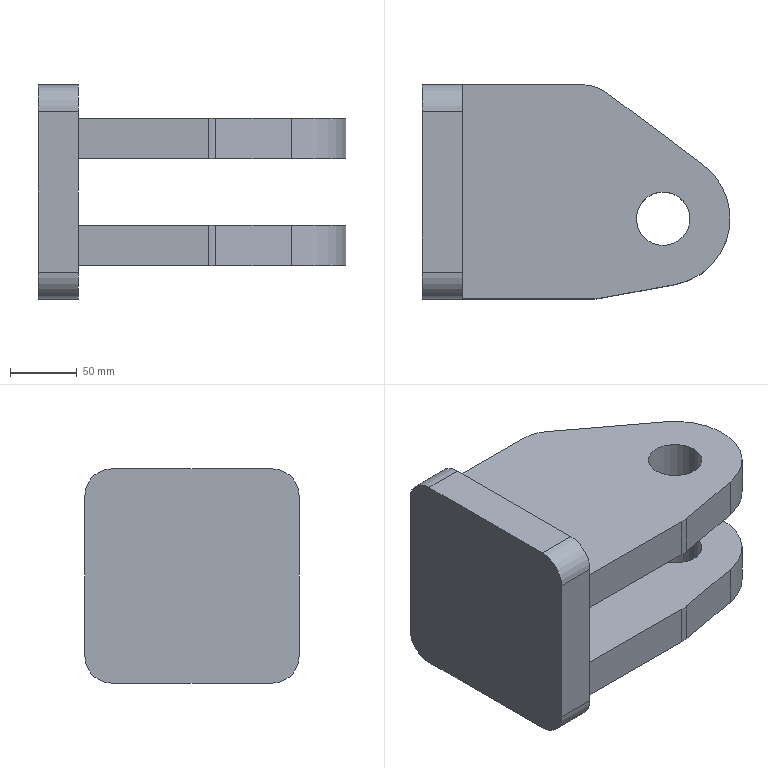Part | SolidWorks | features BaseBody 3 | 3 solids | 34 faces | box 230 x 160 x 160 mm | volume 2295420 mm3 | plane 20 | cylinder 14 | commonest cylinder face diameters 40 x8 60 x4 100 x2
STEP:
#1=CARTESIAN_POINT('',(-15.,60.,-80.));
#2=VERTEX_POINT('',#1);
#3=CARTESIAN_POINT('',(-15.,80.,-60.));
#4=VERTEX_POINT('',#3);
#5=CARTESIAN_POINT('',(-15.,60.,-60.));
#6=DIRECTION('',(1.,0.,0.));
#7=DIRECTION('',(0.,0.,1.));
#8=AXIS2_PLACEMENT_3D('',#5,#6,#7);
#9=CIRCLE('',#8,20.);
#10=EDGE_CURVE('',#2,#4,#9,.T.);
#11=ORIENTED_EDGE('',*,*,#10,.T.);
#12=CARTESIAN_POINT('',(15.,80.,-60.));
#13=VERTEX_POINT('',#12);
#14=CARTESIAN_POINT('',(15.,80.,-60.));
#15=DIRECTION('',(-1.,0.,0.));
#16=VECTOR('',#15,1000.);
#17=LINE('',#14,#16);
#18=EDGE_CURVE('',#13,#4,#17,.T.);
#19=ORIENTED_EDGE('',*,*,#18,.F.);
#20=CARTESIAN_POINT('',(15.,60.,-80.));
#21=VERTEX_POINT('',#20);
#22=CARTESIAN_POINT('',(15.,60.,-60.));
#23=DIRECTION('',(1.,0.,0.));
#24=DIRECTION('',(0.,0.,1.));
#25=AXIS2_PLACEMENT_3D('',#22,#23,#24);
#26=CIRCLE('',#25,20.);
#27=EDGE_CURVE('',#21,#13,#26,.T.);
#28=ORIENTED_EDGE('',*,*,#27,.F.);
#29=CARTESIAN_POINT('',(15.,60.,-80.));
#30=DIRECTION('',(-1.,0.,0.));
#31=VECTOR('',#30,1000.);
#32=LINE('',#29,#31);
#33=EDGE_CURVE('',#21,#2,#32,.T.);
#34=ORIENTED_EDGE('',*,*,#33,.T.);
#35=EDGE_LOOP('',(#11,#19,#28,#34));
#36=FACE_OUTER_BOUND('',#35,.T.);
#37=CARTESIAN_POINT('',(15.,60.,-60.));
#38=DIRECTION('',(-1.,0.,0.));
#39=DIRECTION('',(0.,0.,1.));
#40=AXIS2_PLACEMENT_3D('',#37,#38,#39);
#41=CYLINDRICAL_SURFACE('',#40,20.);
#42=ADVANCED_FACE('',(#36),#41,.T.);
#43=CARTESIAN_POINT('',(-15.,80.,60.));
#44=VERTEX_POINT('',#43);
#45=CARTESIAN_POINT('',(-15.,80.,60.));
#46=DIRECTION('',(0.,0.,1.));
#47=VECTOR('',#46,1000.);
#48=LINE('',#45,#47);
#49=EDGE_CURVE('',#4,#44,#48,.T.);
#50=ORIENTED_EDGE('',*,*,#49,.T.);
#51=CARTESIAN_POINT('',(15.,80.,60.));
#52=VERTEX_POINT('',#51);
#53=CARTESIAN_POINT('',(15.,80.,60.));
#54=DIRECTION('',(-1.,0.,0.));
#55=VECTOR('',#54,1000.);
#56=LINE('',#53,#55);
#57=EDGE_CURVE('',#52,#44,#56,.T.);
#58=ORIENTED_EDGE('',*,*,#57,.F.);
#59=CARTESIAN_POINT('',(15.,80.,60.));
#60=DIRECTION('',(0.,0.,1.));
#61=VECTOR('',#60,1000.);
#62=LINE('',#59,#61);
#63=EDGE_CURVE('',#13,#52,#62,.T.);
#64=ORIENTED_EDGE('',*,*,#63,.F.);
#65=ORIENTED_EDGE('',*,*,#18,.T.);
#66=EDGE_LOOP('',(#50,#58,#64,#65));
#67=FACE_OUTER_BOUND('',#66,.T.);
#68=CARTESIAN_POINT('',(15.,80.,60.));
#69=DIRECTION('',(0.,-1.,0.));
#70=DIRECTION('',(0.,0.,-1.));
#71=AXIS2_PLACEMENT_3D('',#68,#69,#70);
#72=PLANE('',#71);
#73=ADVANCED_FACE('',(#67),#72,.F.);
#74=CARTESIAN_POINT('',(-15.,60.,80.));
#75=VERTEX_POINT('',#74);
#76=CARTESIAN_POINT('',(-15.,60.,60.));
#77=DIRECTION('',(1.,0.,0.));
#78=DIRECTION('',(0.,0.,-1.));
#79=AXIS2_PLACEMENT_3D('',#76,#77,#78);
#80=CIRCLE('',#79,20.);
#81=EDGE_CURVE('',#44,#75,#80,.T.);
#82=ORIENTED_EDGE('',*,*,#81,.T.);
#83=CARTESIAN_POINT('',(15.,60.,80.));
#84=VERTEX_POINT('',#83);
#85=CARTESIAN_POINT('',(15.,60.,80.));
#86=DIRECTION('',(-1.,0.,0.));
#87=VECTOR('',#86,1000.);
#88=LINE('',#85,#87);
#89=EDGE_CURVE('',#84,#75,#88,.T.);
#90=ORIENTED_EDGE('',*,*,#89,.F.);
#91=CARTESIAN_POINT('',(15.,60.,60.));
#92=DIRECTION('',(1.,0.,0.));
#93=DIRECTION('',(0.,0.,-1.));
#94=AXIS2_PLACEMENT_3D('',#91,#92,#93);
#95=CIRCLE('',#94,20.);
#96=EDGE_CURVE('',#52,#84,#95,.T.);
#97=ORIENTED_EDGE('',*,*,#96,.F.);
#98=ORIENTED_EDGE('',*,*,#57,.T.);
#99=EDGE_LOOP('',(#82,#90,#97,#98));
#100=FACE_OUTER_BOUND('',#99,.T.);
#101=CARTESIAN_POINT('',(15.,60.,60.));
#102=DIRECTION('',(-1.,0.,0.));
#103=DIRECTION('',(0.,0.,1.));
#104=AXIS2_PLACEMENT_3D('',#101,#102,#103);
#105=CYLINDRICAL_SURFACE('',#104,20.);
#106=ADVANCED_FACE('',(#100),#105,.T.);
#107=CARTESIAN_POINT('',(-15.,-60.,80.));
#108=VERTEX_POINT('',#107);
#109=CARTESIAN_POINT('',(-15.,60.,80.));
#110=DIRECTION('',(0.,-1.,0.));
#111=VECTOR('',#110,1000.);
#112=LINE('',#109,#111);
#113=EDGE_CURVE('',#75,#108,#112,.T.);
#114=ORIENTED_EDGE('',*,*,#113,.T.);
#115=CARTESIAN_POINT('',(15.,-60.,80.));
#116=VERTEX_POINT('',#115);
#117=CARTESIAN_POINT('',(15.,-60.,80.));
#118=DIRECTION('',(-1.,0.,0.));
#119=VECTOR('',#118,1000.);
#120=LINE('',#117,#119);
#121=EDGE_CURVE('',#116,#108,#120,.T.);
#122=ORIENTED_EDGE('',*,*,#121,.F.);
#123=CARTESIAN_POINT('',(15.,60.,80.));
#124=DIRECTION('',(0.,-1.,0.));
#125=VECTOR('',#124,1000.);
#126=LINE('',#123,#125);
#127=EDGE_CURVE('',#84,#116,#126,.T.);
#128=ORIENTED_EDGE('',*,*,#127,.F.);
#129=ORIENTED_EDGE('',*,*,#89,.T.);
#130=EDGE_LOOP('',(#114,#122,#128,#129));
#131=FACE_OUTER_BOUND('',#130,.T.);
#132=CARTESIAN_POINT('',(15.,60.,80.));
#133=DIRECTION('',(0.,0.,-1.));
#134=DIRECTION('',(-1.,0.,0.));
#135=AXIS2_PLACEMENT_3D('',#132,#133,#134);
#136=PLANE('',#135);
#137=ADVANCED_FACE('',(#131),#136,.F.);
#138=CARTESIAN_POINT('',(-15.,-80.,60.));
#139=VERTEX_POINT('',#138);
#140=CARTESIAN_POINT('',(-15.,-60.,60.));
#141=DIRECTION('',(1.,0.,0.));
#142=DIRECTION('',(0.,0.,-1.));
#143=AXIS2_PLACEMENT_3D('',#140,#141,#142);
#144=CIRCLE('',#143,20.);
#145=EDGE_CURVE('',#108,#139,#144,.T.);
#146=ORIENTED_EDGE('',*,*,#145,.T.);
#147=CARTESIAN_POINT('',(15.,-80.,60.));
#148=VERTEX_POINT('',#147);
#149=CARTESIAN_POINT('',(15.,-80.,60.));
#150=DIRECTION('',(-1.,0.,0.));
#151=VECTOR('',#150,1000.);
#152=LINE('',#149,#151);
#153=EDGE_CURVE('',#148,#139,#152,.T.);
#154=ORIENTED_EDGE('',*,*,#153,.F.);
#155=CARTESIAN_POINT('',(15.,-60.,60.));
#156=DIRECTION('',(1.,0.,0.));
#157=DIRECTION('',(0.,0.,-1.));
#158=AXIS2_PLACEMENT_3D('',#155,#156,#157);
#159=CIRCLE('',#158,20.);
#160=EDGE_CURVE('',#116,#148,#159,.T.);
#161=ORIENTED_EDGE('',*,*,#160,.F.);
#162=ORIENTED_EDGE('',*,*,#121,.T.);
#163=EDGE_LOOP('',(#146,#154,#161,#162));
#164=FACE_OUTER_BOUND('',#163,.T.);
#165=CARTESIAN_POINT('',(15.,-60.,60.));
#166=DIRECTION('',(-1.,0.,0.));
#167=DIRECTION('',(0.,0.,1.));
#168=AXIS2_PLACEMENT_3D('',#165,#166,#167);
#169=CYLINDRICAL_SURFACE('',#168,20.);
#170=ADVANCED_FACE('',(#164),#169,.T.);
#171=CARTESIAN_POINT('',(-15.,-80.,-60.));
#172=VERTEX_POINT('',#171);
#173=CARTESIAN_POINT('',(-15.,-80.,60.));
#174=DIRECTION('',(0.,0.,-1.));
#175=VECTOR('',#174,1000.);
#176=LINE('',#173,#175);
#177=EDGE_CURVE('',#139,#172,#176,.T.);
#178=ORIENTED_EDGE('',*,*,#177,.T.);
#179=CARTESIAN_POINT('',(15.,-80.,-60.));
#180=VERTEX_POINT('',#179);
#181=CARTESIAN_POINT('',(15.,-80.,-60.));
#182=DIRECTION('',(-1.,0.,0.));
#183=VECTOR('',#182,1000.);
#184=LINE('',#181,#183);
#185=EDGE_CURVE('',#180,#172,#184,.T.);
#186=ORIENTED_EDGE('',*,*,#185,.F.);
#187=CARTESIAN_POINT('',(15.,-80.,60.));
#188=DIRECTION('',(0.,0.,-1.));
#189=VECTOR('',#188,1000.);
#190=LINE('',#187,#189);
#191=EDGE_CURVE('',#148,#180,#190,.T.);
#192=ORIENTED_EDGE('',*,*,#191,.F.);
#193=ORIENTED_EDGE('',*,*,#153,.T.);
#194=EDGE_LOOP('',(#178,#186,#192,#193));
#195=FACE_OUTER_BOUND('',#194,.T.);
#196=CARTESIAN_POINT('',(15.,-80.,60.));
#197=DIRECTION('',(0.,1.,0.));
#198=DIRECTION('',(0.,0.,1.));
#199=AXIS2_PLACEMENT_3D('',#196,#197,#198);
#200=PLANE('',#199);
#201=ADVANCED_FACE('',(#195),#200,.F.);
#202=CARTESIAN_POINT('',(-15.,-60.,-80.));
#203=VERTEX_POINT('',#202);
#204=CARTESIAN_POINT('',(-15.,-60.,-60.));
#205=DIRECTION('',(1.,0.,0.));
#206=DIRECTION('',(0.,0.,-1.));
#207=AXIS2_PLACEMENT_3D('',#204,#205,#206);
#208=CIRCLE('',#207,20.);
#209=EDGE_CURVE('',#172,#203,#208,.T.);
#210=ORIENTED_EDGE('',*,*,#209,.T.);
#211=CARTESIAN_POINT('',(15.,-60.,-80.));
#212=VERTEX_POINT('',#211);
#213=CARTESIAN_POINT('',(15.,-60.,-80.));
#214=DIRECTION('',(-1.,0.,0.));
#215=VECTOR('',#214,1000.);
#216=LINE('',#213,#215);
#217=EDGE_CURVE('',#212,#203,#216,.T.);
#218=ORIENTED_EDGE('',*,*,#217,.F.);
#219=CARTESIAN_POINT('',(15.,-60.,-60.));
#220=DIRECTION('',(1.,0.,0.));
#221=DIRECTION('',(0.,0.,-1.));
#222=AXIS2_PLACEMENT_3D('',#219,#220,#221);
#223=CIRCLE('',#222,20.);
#224=EDGE_CURVE('',#180,#212,#223,.T.);
#225=ORIENTED_EDGE('',*,*,#224,.F.);
#226=ORIENTED_EDGE('',*,*,#185,.T.);
#227=EDGE_LOOP('',(#210,#218,#225,#226));
#228=FACE_OUTER_BOUND('',#227,.T.);
#229=CARTESIAN_POINT('',(15.,-60.,-60.));
#230=DIRECTION('',(-1.,0.,0.));
#231=DIRECTION('',(0.,0.,1.));
#232=AXIS2_PLACEMENT_3D('',#229,#230,#231);
#233=CYLINDRICAL_SURFACE('',#232,20.);
#234=ADVANCED_FACE('',(#228),#233,.T.);
#235=CARTESIAN_POINT('',(-15.,60.,-80.));
#236=DIRECTION('',(0.,1.,0.));
#237=VECTOR('',#236,1000.);
#238=LINE('',#235,#237);
#239=EDGE_CURVE('',#203,#2,#238,.T.);
#240=ORIENTED_EDGE('',*,*,#239,.T.);
#241=ORIENTED_EDGE('',*,*,#33,.F.);
#242=CARTESIAN_POINT('',(15.,60.,-80.));
#243=DIRECTION('',(0.,1.,0.));
#244=VECTOR('',#243,1000.);
#245=LINE('',#242,#244);
#246=EDGE_CURVE('',#212,#21,#245,.T.);
#247=ORIENTED_EDGE('',*,*,#246,.F.);
#248=ORIENTED_EDGE('',*,*,#217,.T.);
#249=EDGE_LOOP('',(#240,#241,#247,#248));
#250=FACE_OUTER_BOUND('',#249,.T.);
#251=CARTESIAN_POINT('',(15.,60.,-80.));
#252=DIRECTION('',(0.,0.,1.));
#253=DIRECTION('',(0.,-1.,0.));
#254=AXIS2_PLACEMENT_3D('',#251,#252,#253);
#255=PLANE('',#254);
#256=ADVANCED_FACE('',(#250),#255,.F.);
#257=ORIENTED_EDGE('',*,*,#27,.T.);
#258=ORIENTED_EDGE('',*,*,#63,.T.);
#259=ORIENTED_EDGE('',*,*,#96,.T.);
#260=ORIENTED_EDGE('',*,*,#127,.T.);
#261=ORIENTED_EDGE('',*,*,#160,.T.);
#262=ORIENTED_EDGE('',*,*,#191,.T.);
#263=ORIENTED_EDGE('',*,*,#224,.T.);
#264=ORIENTED_EDGE('',*,*,#246,.T.);
#265=EDGE_LOOP('',(#257,#258,#259,#260,#261,#262,#263,#264));
#266=FACE_OUTER_BOUND('',#265,.T.);
#267=CARTESIAN_POINT('',(15.,60.,-60.));
#268=DIRECTION('',(-1.,0.,0.));
#269=DIRECTION('',(0.,0.,1.));
#270=AXIS2_PLACEMENT_3D('',#267,#268,#269);
#271=PLANE('',#270);
#272=ADVANCED_FACE('',(#266),#271,.F.);
#273=ORIENTED_EDGE('',*,*,#10,.F.);
#274=ORIENTED_EDGE('',*,*,#239,.F.);
#275=ORIENTED_EDGE('',*,*,#209,.F.);
#276=ORIENTED_EDGE('',*,*,#177,.F.);
#277=ORIENTED_EDGE('',*,*,#145,.F.);
#278=ORIENTED_EDGE('',*,*,#113,.F.);
#279=ORIENTED_EDGE('',*,*,#81,.F.);
#280=ORIENTED_EDGE('',*,*,#49,.F.);
#281=EDGE_LOOP('',(#273,#274,#275,#276,#277,#278,#279,#280));
#282=FACE_OUTER_BOUND('',#281,.T.);
#283=CARTESIAN_POINT('',(-15.,60.,-60.));
#284=DIRECTION('',(-1.,0.,0.));
#285=DIRECTION('',(0.,0.,1.));
#286=AXIS2_PLACEMENT_3D('',#283,#284,#285);
#287=PLANE('',#286);
#288=ADVANCED_FACE('',(#282),#287,.T.);
#289=CLOSED_SHELL('',(#42,#73,#106,#137,#170,#201,#234,#256,#272,#288));
#290=MANIFOLD_SOLID_BREP('',#289);
#291=CARTESIAN_POINT('',(145.,-20.,55.));
#292=VERTEX_POINT('',#291);
#293=CARTESIAN_POINT('',(185.,-20.,55.));
#294=VERTEX_POINT('',#293);
#295=CARTESIAN_POINT('',(165.,-20.,55.));
#296=DIRECTION('',(0.,0.,1.));
#297=DIRECTION('',(1.,0.,0.));
#298=AXIS2_PLACEMENT_3D('',#295,#296,#297);
#299=CIRCLE('',#298,20.);
#300=EDGE_CURVE('',#292,#294,#299,.T.);
#301=ORIENTED_EDGE('',*,*,#300,.T.);
#302=CARTESIAN_POINT('',(185.,-20.,25.));
#303=VERTEX_POINT('',#302);
#304=CARTESIAN_POINT('',(185.,-20.,55.));
#305=DIRECTION('',(0.,0.,-1.));
#306=VECTOR('',#305,1000.);
#307=LINE('',#304,#306);
#308=EDGE_CURVE('',#294,#303,#307,.T.);
#309=ORIENTED_EDGE('',*,*,#308,.T.);
#310=CARTESIAN_POINT('',(145.,-20.,25.));
#311=VERTEX_POINT('',#310);
#312=CARTESIAN_POINT('',(165.,-20.,25.));
#313=DIRECTION('',(0.,0.,1.));
#314=DIRECTION('',(1.,0.,0.));
#315=AXIS2_PLACEMENT_3D('',#312,#313,#314);
#316=CIRCLE('',#315,20.);
#317=EDGE_CURVE('',#311,#303,#316,.T.);
#318=ORIENTED_EDGE('',*,*,#317,.F.);
#319=CARTESIAN_POINT('',(145.,-20.,55.));
#320=DIRECTION('',(0.,0.,-1.));
#321=VECTOR('',#320,1000.);
#322=LINE('',#319,#321);
#323=EDGE_CURVE('',#292,#311,#322,.T.);
#324=ORIENTED_EDGE('',*,*,#323,.F.);
#325=EDGE_LOOP('',(#301,#309,#318,#324));
#326=FACE_OUTER_BOUND('',#325,.T.);
#327=CARTESIAN_POINT('',(165.,-20.,55.));
#328=DIRECTION('',(0.,0.,-1.));
#329=DIRECTION('',(-1.,0.,0.));
#330=AXIS2_PLACEMENT_3D('',#327,#328,#329);
#331=CYLINDRICAL_SURFACE('',#330,20.);
#332=ADVANCED_FACE('',(#326),#331,.F.);
#333=CARTESIAN_POINT('',(15.,80.,55.));
#334=VERTEX_POINT('',#333);
#335=CARTESIAN_POINT('',(15.,-80.,55.));
#336=VERTEX_POINT('',#335);
#337=CARTESIAN_POINT('',(15.,80.,55.));
#338=DIRECTION('',(0.,-1.,0.));
#339=VECTOR('',#338,1000.);
#340=LINE('',#337,#339);
#341=EDGE_CURVE('',#334,#336,#340,.T.);
#342=ORIENTED_EDGE('',*,*,#341,.T.);
#343=CARTESIAN_POINT('',(112.273,-80.,55.));
#344=VERTEX_POINT('',#343);
#345=CARTESIAN_POINT('',(15.,-80.,55.));
#346=DIRECTION('',(1.,0.,0.));
#347=VECTOR('',#346,1000.);
#348=LINE('',#345,#347);
#349=EDGE_CURVE('',#336,#344,#348,.T.);
#350=ORIENTED_EDGE('',*,*,#349,.T.);
#351=CARTESIAN_POINT('',(117.683,-79.508,55.));
#352=VERTEX_POINT('',#351);
#353=CARTESIAN_POINT('',(112.273,-50.,55.));
#354=DIRECTION('',(0.,0.,1.));
#355=DIRECTION('',(1.,0.,0.));
#356=AXIS2_PLACEMENT_3D('',#353,#354,#355);
#357=CIRCLE('',#356,30.);
#358=EDGE_CURVE('',#344,#352,#357,.T.);
#359=ORIENTED_EDGE('',*,*,#358,.T.);
#360=CARTESIAN_POINT('',(174.016,-69.18,55.));
#361=VERTEX_POINT('',#360);
#362=CARTESIAN_POINT('',(117.683,-79.508,55.));
#363=DIRECTION('',(0.9836,0.1803,0.));
#364=VECTOR('',#363,1000.);
#365=LINE('',#362,#364);
#366=EDGE_CURVE('',#352,#361,#365,.T.);
#367=ORIENTED_EDGE('',*,*,#366,.T.);
#368=CARTESIAN_POINT('',(195.,20.,55.));
#369=VERTEX_POINT('',#368);
#370=CARTESIAN_POINT('',(165.,-20.,55.));
#371=DIRECTION('',(0.,0.,1.));
#372=DIRECTION('',(1.,0.,0.));
#373=AXIS2_PLACEMENT_3D('',#370,#371,#372);
#374=CIRCLE('',#373,50.);
#375=EDGE_CURVE('',#361,#369,#374,.T.);
#376=ORIENTED_EDGE('',*,*,#375,.T.);
#377=CARTESIAN_POINT('',(123.,74.,55.));
#378=VERTEX_POINT('',#377);
#379=CARTESIAN_POINT('',(123.,74.,55.));
#380=DIRECTION('',(-0.8,0.6,0.));
#381=VECTOR('',#380,1000.);
#382=LINE('',#379,#381);
#383=EDGE_CURVE('',#369,#378,#382,.T.);
#384=ORIENTED_EDGE('',*,*,#383,.T.);
#385=CARTESIAN_POINT('',(105.,80.,55.));
#386=VERTEX_POINT('',#385);
#387=CARTESIAN_POINT('',(105.,50.,55.));
#388=DIRECTION('',(0.,0.,1.));
#389=DIRECTION('',(-1.,0.,0.));
#390=AXIS2_PLACEMENT_3D('',#387,#388,#389);
#391=CIRCLE('',#390,30.);
#392=EDGE_CURVE('',#378,#386,#391,.T.);
#393=ORIENTED_EDGE('',*,*,#392,.T.);
#394=CARTESIAN_POINT('',(15.,80.,55.));
#395=DIRECTION('',(-1.,0.,0.));
#396=VECTOR('',#395,1000.);
#397=LINE('',#394,#396);
#398=EDGE_CURVE('',#386,#334,#397,.T.);
#399=ORIENTED_EDGE('',*,*,#398,.T.);
#400=EDGE_LOOP('',(#342,#350,#359,#367,#376,#384,#393,#399));
#401=FACE_OUTER_BOUND('',#400,.T.);
#402=ORIENTED_EDGE('',*,*,#300,.F.);
#403=CARTESIAN_POINT('',(165.,-20.,55.));
#404=DIRECTION('',(0.,0.,1.));
#405=DIRECTION('',(1.,0.,0.));
#406=AXIS2_PLACEMENT_3D('',#403,#404,#405);
#407=CIRCLE('',#406,20.);
#408=EDGE_CURVE('',#294,#292,#407,.T.);
#409=ORIENTED_EDGE('',*,*,#408,.F.);
#410=EDGE_LOOP('',(#402,#409));
#411=FACE_BOUND('',#410,.T.);
#412=CARTESIAN_POINT('',(112.273,-50.,55.));
#413=DIRECTION('',(0.,0.,1.));
#414=DIRECTION('',(1.,0.,0.));
#415=AXIS2_PLACEMENT_3D('',#412,#413,#414);
#416=PLANE('',#415);
#417=ADVANCED_FACE('',(#401,#411),#416,.T.);
#418=CARTESIAN_POINT('',(15.,80.,25.));
#419=VERTEX_POINT('',#418);
#420=CARTESIAN_POINT('',(15.,-80.,25.));
#421=VERTEX_POINT('',#420);
#422=CARTESIAN_POINT('',(15.,80.,25.));
#423=DIRECTION('',(0.,-1.,0.));
#424=VECTOR('',#423,1000.);
#425=LINE('',#422,#424);
#426=EDGE_CURVE('',#419,#421,#425,.T.);
#427=ORIENTED_EDGE('',*,*,#426,.F.);
#428=CARTESIAN_POINT('',(105.,80.,25.));
#429=VERTEX_POINT('',#428);
#430=CARTESIAN_POINT('',(15.,80.,25.));
#431=DIRECTION('',(-1.,0.,0.));
#432=VECTOR('',#431,1000.);
#433=LINE('',#430,#432);
#434=EDGE_CURVE('',#429,#419,#433,.T.);
#435=ORIENTED_EDGE('',*,*,#434,.F.);
#436=CARTESIAN_POINT('',(123.,74.,25.));
#437=VERTEX_POINT('',#436);
#438=CARTESIAN_POINT('',(105.,50.,25.));
#439=DIRECTION('',(0.,0.,1.));
#440=DIRECTION('',(-1.,0.,0.));
#441=AXIS2_PLACEMENT_3D('',#438,#439,#440);
#442=CIRCLE('',#441,30.);
#443=EDGE_CURVE('',#437,#429,#442,.T.);
#444=ORIENTED_EDGE('',*,*,#443,.F.);
#445=CARTESIAN_POINT('',(195.,20.,25.));
#446=VERTEX_POINT('',#445);
#447=CARTESIAN_POINT('',(123.,74.,25.));
#448=DIRECTION('',(-0.8,0.6,0.));
#449=VECTOR('',#448,1000.);
#450=LINE('',#447,#449);
#451=EDGE_CURVE('',#446,#437,#450,.T.);
#452=ORIENTED_EDGE('',*,*,#451,.F.);
#453=CARTESIAN_POINT('',(174.016,-69.18,25.));
#454=VERTEX_POINT('',#453);
#455=CARTESIAN_POINT('',(165.,-20.,25.));
#456=DIRECTION('',(0.,0.,1.));
#457=DIRECTION('',(1.,0.,0.));
#458=AXIS2_PLACEMENT_3D('',#455,#456,#457);
#459=CIRCLE('',#458,50.);
#460=EDGE_CURVE('',#454,#446,#459,.T.);
#461=ORIENTED_EDGE('',*,*,#460,.F.);
#462=CARTESIAN_POINT('',(117.683,-79.508,25.));
#463=VERTEX_POINT('',#462);
#464=CARTESIAN_POINT('',(117.683,-79.508,25.));
#465=DIRECTION('',(0.9836,0.1803,0.));
#466=VECTOR('',#465,1000.);
#467=LINE('',#464,#466);
#468=EDGE_CURVE('',#463,#454,#467,.T.);
#469=ORIENTED_EDGE('',*,*,#468,.F.);
#470=CARTESIAN_POINT('',(112.273,-80.,25.));
#471=VERTEX_POINT('',#470);
#472=CARTESIAN_POINT('',(112.273,-50.,25.));
#473=DIRECTION('',(0.,0.,1.));
#474=DIRECTION('',(1.,0.,0.));
#475=AXIS2_PLACEMENT_3D('',#472,#473,#474);
#476=CIRCLE('',#475,30.);
#477=EDGE_CURVE('',#471,#463,#476,.T.);
#478=ORIENTED_EDGE('',*,*,#477,.F.);
#479=CARTESIAN_POINT('',(15.,-80.,25.));
#480=DIRECTION('',(1.,0.,0.));
#481=VECTOR('',#480,1000.);
#482=LINE('',#479,#481);
#483=EDGE_CURVE('',#421,#471,#482,.T.);
#484=ORIENTED_EDGE('',*,*,#483,.F.);
#485=EDGE_LOOP('',(#427,#435,#444,#452,#461,#469,#478,#484));
#486=FACE_OUTER_BOUND('',#485,.T.);
#487=ORIENTED_EDGE('',*,*,#317,.T.);
#488=CARTESIAN_POINT('',(165.,-20.,25.));
#489=DIRECTION('',(0.,0.,1.));
#490=DIRECTION('',(1.,0.,0.));
#491=AXIS2_PLACEMENT_3D('',#488,#489,#490);
#492=CIRCLE('',#491,20.);
#493=EDGE_CURVE('',#303,#311,#492,.T.);
#494=ORIENTED_EDGE('',*,*,#493,.T.);
#495=EDGE_LOOP('',(#487,#494));
#496=FACE_BOUND('',#495,.T.);
#497=CARTESIAN_POINT('',(112.273,-50.,25.));
#498=DIRECTION('',(0.,0.,1.));
#499=DIRECTION('',(1.,0.,0.));
#500=AXIS2_PLACEMENT_3D('',#497,#498,#499);
#501=PLANE('',#500);
#502=ADVANCED_FACE('',(#486,#496),#501,.F.);
#503=ORIENTED_EDGE('',*,*,#426,.T.);
#504=CARTESIAN_POINT('',(15.,-80.,55.));
#505=DIRECTION('',(0.,0.,-1.));
#506=VECTOR('',#505,1000.);
#507=LINE('',#504,#506);
#508=EDGE_CURVE('',#336,#421,#507,.T.);
#509=ORIENTED_EDGE('',*,*,#508,.F.);
#510=ORIENTED_EDGE('',*,*,#341,.F.);
#511=CARTESIAN_POINT('',(15.,80.,55.));
#512=DIRECTION('',(0.,0.,-1.));
#513=VECTOR('',#512,1000.);
#514=LINE('',#511,#513);
#515=EDGE_CURVE('',#334,#419,#514,.T.);
#516=ORIENTED_EDGE('',*,*,#515,.T.);
#517=EDGE_LOOP('',(#503,#509,#510,#516));
#518=FACE_OUTER_BOUND('',#517,.T.);
#519=CARTESIAN_POINT('',(15.,80.,55.));
#520=DIRECTION('',(1.,0.,0.));
#521=DIRECTION('',(0.,0.,-1.));
#522=AXIS2_PLACEMENT_3D('',#519,#520,#521);
#523=PLANE('',#522);
#524=ADVANCED_FACE('',(#518),#523,.F.);
#525=ORIENTED_EDGE('',*,*,#483,.T.);
#526=CARTESIAN_POINT('',(112.273,-80.,55.));
#527=DIRECTION('',(0.,0.,-1.));
#528=VECTOR('',#527,1000.);
#529=LINE('',#526,#528);
#530=EDGE_CURVE('',#344,#471,#529,.T.);
#531=ORIENTED_EDGE('',*,*,#530,.F.);
#532=ORIENTED_EDGE('',*,*,#349,.F.);
#533=ORIENTED_EDGE('',*,*,#508,.T.);
#534=EDGE_LOOP('',(#525,#531,#532,#533));
#535=FACE_OUTER_BOUND('',#534,.T.);
#536=CARTESIAN_POINT('',(15.,-80.,55.));
#537=DIRECTION('',(0.,1.,0.));
#538=DIRECTION('',(-1.,0.,0.));
#539=AXIS2_PLACEMENT_3D('',#536,#537,#538);
#540=PLANE('',#539);
#541=ADVANCED_FACE('',(#535),#540,.F.);
#542=ORIENTED_EDGE('',*,*,#477,.T.);
#543=CARTESIAN_POINT('',(117.683,-79.508,55.));
#544=DIRECTION('',(0.,0.,-1.));
#545=VECTOR('',#544,1000.);
#546=LINE('',#543,#545);
#547=EDGE_CURVE('',#352,#463,#546,.T.);
#548=ORIENTED_EDGE('',*,*,#547,.F.);
#549=ORIENTED_EDGE('',*,*,#358,.F.);
#550=ORIENTED_EDGE('',*,*,#530,.T.);
#551=EDGE_LOOP('',(#542,#548,#549,#550));
#552=FACE_OUTER_BOUND('',#551,.T.);
#553=CARTESIAN_POINT('',(112.273,-50.,55.));
#554=DIRECTION('',(0.,0.,-1.));
#555=DIRECTION('',(-1.,0.,0.));
#556=AXIS2_PLACEMENT_3D('',#553,#554,#555);
#557=CYLINDRICAL_SURFACE('',#556,30.);
#558=ADVANCED_FACE('',(#552),#557,.T.);
#559=ORIENTED_EDGE('',*,*,#468,.T.);
#560=CARTESIAN_POINT('',(174.016,-69.18,55.));
#561=DIRECTION('',(0.,0.,-1.));
#562=VECTOR('',#561,1000.);
#563=LINE('',#560,#562);
#564=EDGE_CURVE('',#361,#454,#563,.T.);
#565=ORIENTED_EDGE('',*,*,#564,.F.);
#566=ORIENTED_EDGE('',*,*,#366,.F.);
#567=ORIENTED_EDGE('',*,*,#547,.T.);
#568=EDGE_LOOP('',(#559,#565,#566,#567));
#569=FACE_OUTER_BOUND('',#568,.T.);
#570=CARTESIAN_POINT('',(117.683,-79.508,55.));
#571=DIRECTION('',(-0.1803,0.9836,0.));
#572=DIRECTION('',(-0.9836,-0.1803,0.));
#573=AXIS2_PLACEMENT_3D('',#570,#571,#572);
#574=PLANE('',#573);
#575=ADVANCED_FACE('',(#569),#574,.F.);
#576=ORIENTED_EDGE('',*,*,#460,.T.);
#577=CARTESIAN_POINT('',(195.,20.,55.));
#578=DIRECTION('',(0.,0.,-1.));
#579=VECTOR('',#578,1000.);
#580=LINE('',#577,#579);
#581=EDGE_CURVE('',#369,#446,#580,.T.);
#582=ORIENTED_EDGE('',*,*,#581,.F.);
#583=ORIENTED_EDGE('',*,*,#375,.F.);
#584=ORIENTED_EDGE('',*,*,#564,.T.);
#585=EDGE_LOOP('',(#576,#582,#583,#584));
#586=FACE_OUTER_BOUND('',#585,.T.);
#587=CARTESIAN_POINT('',(165.,-20.,55.));
#588=DIRECTION('',(0.,0.,-1.));
#589=DIRECTION('',(-1.,0.,0.));
#590=AXIS2_PLACEMENT_3D('',#587,#588,#589);
#591=CYLINDRICAL_SURFACE('',#590,50.);
#592=ADVANCED_FACE('',(#586),#591,.T.);
#593=ORIENTED_EDGE('',*,*,#451,.T.);
#594=CARTESIAN_POINT('',(123.,74.,55.));
#595=DIRECTION('',(0.,0.,-1.));
#596=VECTOR('',#595,1000.);
#597=LINE('',#594,#596);
#598=EDGE_CURVE('',#378,#437,#597,.T.);
#599=ORIENTED_EDGE('',*,*,#598,.F.);
#600=ORIENTED_EDGE('',*,*,#383,.F.);
#601=ORIENTED_EDGE('',*,*,#581,.T.);
#602=EDGE_LOOP('',(#593,#599,#600,#601));
#603=FACE_OUTER_BOUND('',#602,.T.);
#604=CARTESIAN_POINT('',(123.,74.,55.));
#605=DIRECTION('',(-0.6,-0.8,0.));
#606=DIRECTION('',(0.8,-0.6,0.));
#607=AXIS2_PLACEMENT_3D('',#604,#605,#606);
#608=PLANE('',#607);
#609=ADVANCED_FACE('',(#603),#608,.F.);
#610=ORIENTED_EDGE('',*,*,#443,.T.);
#611=CARTESIAN_POINT('',(105.,80.,55.));
#612=DIRECTION('',(0.,0.,-1.));
#613=VECTOR('',#612,1000.);
#614=LINE('',#611,#613);
#615=EDGE_CURVE('',#386,#429,#614,.T.);
#616=ORIENTED_EDGE('',*,*,#615,.F.);
#617=ORIENTED_EDGE('',*,*,#392,.F.);
#618=ORIENTED_EDGE('',*,*,#598,.T.);
#619=EDGE_LOOP('',(#610,#616,#617,#618));
#620=FACE_OUTER_BOUND('',#619,.T.);
#621=CARTESIAN_POINT('',(105.,50.,55.));
#622=DIRECTION('',(0.,0.,-1.));
#623=DIRECTION('',(-1.,0.,0.));
#624=AXIS2_PLACEMENT_3D('',#621,#622,#623);
#625=CYLINDRICAL_SURFACE('',#624,30.);
#626=ADVANCED_FACE('',(#620),#625,.T.);
#627=ORIENTED_EDGE('',*,*,#434,.T.);
#628=ORIENTED_EDGE('',*,*,#515,.F.);
#629=ORIENTED_EDGE('',*,*,#398,.F.);
#630=ORIENTED_EDGE('',*,*,#615,.T.);
#631=EDGE_LOOP('',(#627,#628,#629,#630));
#632=FACE_OUTER_BOUND('',#631,.T.);
#633=CARTESIAN_POINT('',(15.,80.,55.));
#634=DIRECTION('',(0.,-1.,0.));
#635=DIRECTION('',(1.,0.,0.));
#636=AXIS2_PLACEMENT_3D('',#633,#634,#635);
#637=PLANE('',#636);
#638=ADVANCED_FACE('',(#632),#637,.F.);
#639=ORIENTED_EDGE('',*,*,#308,.F.);
#640=ORIENTED_EDGE('',*,*,#408,.T.);
#641=ORIENTED_EDGE('',*,*,#323,.T.);
#642=ORIENTED_EDGE('',*,*,#493,.F.);
#643=EDGE_LOOP('',(#639,#640,#641,#642));
#644=FACE_OUTER_BOUND('',#643,.T.);
#645=CARTESIAN_POINT('',(165.,-20.,55.));
#646=DIRECTION('',(0.,0.,-1.));
#647=DIRECTION('',(-1.,0.,0.));
#648=AXIS2_PLACEMENT_3D('',#645,#646,#647);
#649=CYLINDRICAL_SURFACE('',#648,20.);
#650=ADVANCED_FACE('',(#644),#649,.F.);
#651=CLOSED_SHELL('',(#332,#417,#502,#524,#541,#558,#575,#592,#609,#626,#638,#650));
#652=MANIFOLD_SOLID_BREP('',#651);
#653=CARTESIAN_POINT('',(185.,-20.,-55.));
#654=VERTEX_POINT('',#653);
#655=CARTESIAN_POINT('',(145.,-20.,-55.));
#656=VERTEX_POINT('',#655);
#657=CARTESIAN_POINT('',(165.,-20.,-55.));
#658=DIRECTION('',(0.,0.,1.));
#659=DIRECTION('',(1.,0.,0.));
#660=AXIS2_PLACEMENT_3D('',#657,#658,#659);
#661=CIRCLE('',#660,20.);
#662=EDGE_CURVE('',#654,#656,#661,.T.);
#663=ORIENTED_EDGE('',*,*,#662,.F.);
#664=CARTESIAN_POINT('',(185.,-20.,-25.));
#665=VERTEX_POINT('',#664);
#666=CARTESIAN_POINT('',(185.,-20.,-55.));
#667=DIRECTION('',(0.,0.,1.));
#668=VECTOR('',#667,1000.);
#669=LINE('',#666,#668);
#670=EDGE_CURVE('',#654,#665,#669,.T.);
#671=ORIENTED_EDGE('',*,*,#670,.T.);
#672=CARTESIAN_POINT('',(145.,-20.,-25.));
#673=VERTEX_POINT('',#672);
#674=CARTESIAN_POINT('',(165.,-20.,-25.));
#675=DIRECTION('',(0.,0.,1.));
#676=DIRECTION('',(1.,0.,0.));
#677=AXIS2_PLACEMENT_3D('',#674,#675,#676);
#678=CIRCLE('',#677,20.);
#679=EDGE_CURVE('',#665,#673,#678,.T.);
#680=ORIENTED_EDGE('',*,*,#679,.T.);
#681=CARTESIAN_POINT('',(145.,-20.,-55.));
#682=DIRECTION('',(0.,0.,1.));
#683=VECTOR('',#682,1000.);
#684=LINE('',#681,#683);
#685=EDGE_CURVE('',#656,#673,#684,.T.);
#686=ORIENTED_EDGE('',*,*,#685,.F.);
#687=EDGE_LOOP('',(#663,#671,#680,#686));
#688=FACE_OUTER_BOUND('',#687,.T.);
#689=CARTESIAN_POINT('',(165.,-20.,-55.));
#690=DIRECTION('',(0.,0.,1.));
#691=DIRECTION('',(-1.,0.,0.));
#692=AXIS2_PLACEMENT_3D('',#689,#690,#691);
#693=CYLINDRICAL_SURFACE('',#692,20.);
#694=ADVANCED_FACE('',(#688),#693,.F.);
#695=CARTESIAN_POINT('',(15.,80.,-55.));
#696=VERTEX_POINT('',#695);
#697=CARTESIAN_POINT('',(15.,-80.,-55.));
#698=VERTEX_POINT('',#697);
#699=CARTESIAN_POINT('',(15.,80.,-55.));
#700=DIRECTION('',(0.,-1.,0.));
#701=VECTOR('',#700,1000.);
#702=LINE('',#699,#701);
#703=EDGE_CURVE('',#696,#698,#702,.T.);
#704=ORIENTED_EDGE('',*,*,#703,.F.);
#705=CARTESIAN_POINT('',(105.,80.,-55.));
#706=VERTEX_POINT('',#705);
#707=CARTESIAN_POINT('',(15.,80.,-55.));
#708=DIRECTION('',(-1.,0.,0.));
#709=VECTOR('',#708,1000.);
#710=LINE('',#707,#709);
#711=EDGE_CURVE('',#706,#696,#710,.T.);
#712=ORIENTED_EDGE('',*,*,#711,.F.);
#713=CARTESIAN_POINT('',(123.,74.,-55.));
#714=VERTEX_POINT('',#713);
#715=CARTESIAN_POINT('',(105.,50.,-55.));
#716=DIRECTION('',(0.,0.,1.));
#717=DIRECTION('',(-1.,0.,0.));
#718=AXIS2_PLACEMENT_3D('',#715,#716,#717);
#719=CIRCLE('',#718,30.);
#720=EDGE_CURVE('',#714,#706,#719,.T.);
#721=ORIENTED_EDGE('',*,*,#720,.F.);
#722=CARTESIAN_POINT('',(195.,20.,-55.));
#723=VERTEX_POINT('',#722);
#724=CARTESIAN_POINT('',(123.,74.,-55.));
#725=DIRECTION('',(-0.8,0.6,0.));
#726=VECTOR('',#725,1000.);
#727=LINE('',#724,#726);
#728=EDGE_CURVE('',#723,#714,#727,.T.);
#729=ORIENTED_EDGE('',*,*,#728,.F.);
#730=CARTESIAN_POINT('',(174.016,-69.18,-55.));
#731=VERTEX_POINT('',#730);
#732=CARTESIAN_POINT('',(165.,-20.,-55.));
#733=DIRECTION('',(0.,0.,1.));
#734=DIRECTION('',(1.,0.,0.));
#735=AXIS2_PLACEMENT_3D('',#732,#733,#734);
#736=CIRCLE('',#735,50.);
#737=EDGE_CURVE('',#731,#723,#736,.T.);
#738=ORIENTED_EDGE('',*,*,#737,.F.);
#739=CARTESIAN_POINT('',(117.683,-79.508,-55.));
#740=VERTEX_POINT('',#739);
#741=CARTESIAN_POINT('',(117.683,-79.508,-55.));
#742=DIRECTION('',(0.9836,0.1803,0.));
#743=VECTOR('',#742,1000.);
#744=LINE('',#741,#743);
#745=EDGE_CURVE('',#740,#731,#744,.T.);
#746=ORIENTED_EDGE('',*,*,#745,.F.);
#747=CARTESIAN_POINT('',(112.273,-80.,-55.));
#748=VERTEX_POINT('',#747);
#749=CARTESIAN_POINT('',(112.273,-50.,-55.));
#750=DIRECTION('',(0.,0.,1.));
#751=DIRECTION('',(1.,0.,0.));
#752=AXIS2_PLACEMENT_3D('',#749,#750,#751);
#753=CIRCLE('',#752,30.);
#754=EDGE_CURVE('',#748,#740,#753,.T.);
#755=ORIENTED_EDGE('',*,*,#754,.F.);
#756=CARTESIAN_POINT('',(15.,-80.,-55.));
#757=DIRECTION('',(1.,0.,0.));
#758=VECTOR('',#757,1000.);
#759=LINE('',#756,#758);
#760=EDGE_CURVE('',#698,#748,#759,.T.);
#761=ORIENTED_EDGE('',*,*,#760,.F.);
#762=EDGE_LOOP('',(#704,#712,#721,#729,#738,#746,#755,#761));
#763=FACE_OUTER_BOUND('',#762,.T.);
#764=CARTESIAN_POINT('',(165.,-20.,-55.));
#765=DIRECTION('',(0.,0.,1.));
#766=DIRECTION('',(1.,0.,0.));
#767=AXIS2_PLACEMENT_3D('',#764,#765,#766);
#768=CIRCLE('',#767,20.);
#769=EDGE_CURVE('',#656,#654,#768,.T.);
#770=ORIENTED_EDGE('',*,*,#769,.T.);
#771=ORIENTED_EDGE('',*,*,#662,.T.);
#772=EDGE_LOOP('',(#770,#771));
#773=FACE_BOUND('',#772,.T.);
#774=CARTESIAN_POINT('',(112.273,-50.,-55.));
#775=DIRECTION('',(0.,0.,-1.));
#776=DIRECTION('',(1.,0.,0.));
#777=AXIS2_PLACEMENT_3D('',#774,#775,#776);
#778=PLANE('',#777);
#779=ADVANCED_FACE('',(#763,#773),#778,.T.);
#780=CARTESIAN_POINT('',(15.,80.,-25.));
#781=VERTEX_POINT('',#780);
#782=CARTESIAN_POINT('',(15.,-80.,-25.));
#783=VERTEX_POINT('',#782);
#784=CARTESIAN_POINT('',(15.,80.,-25.));
#785=DIRECTION('',(0.,-1.,0.));
#786=VECTOR('',#785,1000.);
#787=LINE('',#784,#786);
#788=EDGE_CURVE('',#781,#783,#787,.T.);
#789=ORIENTED_EDGE('',*,*,#788,.T.);
#790=CARTESIAN_POINT('',(112.273,-80.,-25.));
#791=VERTEX_POINT('',#790);
#792=CARTESIAN_POINT('',(15.,-80.,-25.));
#793=DIRECTION('',(1.,0.,0.));
#794=VECTOR('',#793,1000.);
#795=LINE('',#792,#794);
#796=EDGE_CURVE('',#783,#791,#795,.T.);
#797=ORIENTED_EDGE('',*,*,#796,.T.);
#798=CARTESIAN_POINT('',(117.683,-79.508,-25.));
#799=VERTEX_POINT('',#798);
#800=CARTESIAN_POINT('',(112.273,-50.,-25.));
#801=DIRECTION('',(0.,0.,1.));
#802=DIRECTION('',(1.,0.,0.));
#803=AXIS2_PLACEMENT_3D('',#800,#801,#802);
#804=CIRCLE('',#803,30.);
#805=EDGE_CURVE('',#791,#799,#804,.T.);
#806=ORIENTED_EDGE('',*,*,#805,.T.);
#807=CARTESIAN_POINT('',(174.016,-69.18,-25.));
#808=VERTEX_POINT('',#807);
#809=CARTESIAN_POINT('',(117.683,-79.508,-25.));
#810=DIRECTION('',(0.9836,0.1803,0.));
#811=VECTOR('',#810,1000.);
#812=LINE('',#809,#811);
#813=EDGE_CURVE('',#799,#808,#812,.T.);
#814=ORIENTED_EDGE('',*,*,#813,.T.);
#815=CARTESIAN_POINT('',(195.,20.,-25.));
#816=VERTEX_POINT('',#815);
#817=CARTESIAN_POINT('',(165.,-20.,-25.));
#818=DIRECTION('',(0.,0.,1.));
#819=DIRECTION('',(1.,0.,0.));
#820=AXIS2_PLACEMENT_3D('',#817,#818,#819);
#821=CIRCLE('',#820,50.);
#822=EDGE_CURVE('',#808,#816,#821,.T.);
#823=ORIENTED_EDGE('',*,*,#822,.T.);
#824=CARTESIAN_POINT('',(123.,74.,-25.));
#825=VERTEX_POINT('',#824);
#826=CARTESIAN_POINT('',(123.,74.,-25.));
#827=DIRECTION('',(-0.8,0.6,0.));
#828=VECTOR('',#827,1000.);
#829=LINE('',#826,#828);
#830=EDGE_CURVE('',#816,#825,#829,.T.);
#831=ORIENTED_EDGE('',*,*,#830,.T.);
#832=CARTESIAN_POINT('',(105.,80.,-25.));
#833=VERTEX_POINT('',#832);
#834=CARTESIAN_POINT('',(105.,50.,-25.));
#835=DIRECTION('',(0.,0.,1.));
#836=DIRECTION('',(-1.,0.,0.));
#837=AXIS2_PLACEMENT_3D('',#834,#835,#836);
#838=CIRCLE('',#837,30.);
#839=EDGE_CURVE('',#825,#833,#838,.T.);
#840=ORIENTED_EDGE('',*,*,#839,.T.);
#841=CARTESIAN_POINT('',(15.,80.,-25.));
#842=DIRECTION('',(-1.,0.,0.));
#843=VECTOR('',#842,1000.);
#844=LINE('',#841,#843);
#845=EDGE_CURVE('',#833,#781,#844,.T.);
#846=ORIENTED_EDGE('',*,*,#845,.T.);
#847=EDGE_LOOP('',(#789,#797,#806,#814,#823,#831,#840,#846));
#848=FACE_OUTER_BOUND('',#847,.T.);
#849=CARTESIAN_POINT('',(165.,-20.,-25.));
#850=DIRECTION('',(0.,0.,1.));
#851=DIRECTION('',(1.,0.,0.));
#852=AXIS2_PLACEMENT_3D('',#849,#850,#851);
#853=CIRCLE('',#852,20.);
#854=EDGE_CURVE('',#673,#665,#853,.T.);
#855=ORIENTED_EDGE('',*,*,#854,.F.);
#856=ORIENTED_EDGE('',*,*,#679,.F.);
#857=EDGE_LOOP('',(#855,#856));
#858=FACE_BOUND('',#857,.T.);
#859=CARTESIAN_POINT('',(112.273,-50.,-25.));
#860=DIRECTION('',(0.,0.,-1.));
#861=DIRECTION('',(1.,0.,0.));
#862=AXIS2_PLACEMENT_3D('',#859,#860,#861);
#863=PLANE('',#862);
#864=ADVANCED_FACE('',(#848,#858),#863,.F.);
#865=ORIENTED_EDGE('',*,*,#788,.F.);
#866=CARTESIAN_POINT('',(15.,80.,-55.));
#867=DIRECTION('',(0.,0.,1.));
#868=VECTOR('',#867,1000.);
#869=LINE('',#866,#868);
#870=EDGE_CURVE('',#696,#781,#869,.T.);
#871=ORIENTED_EDGE('',*,*,#870,.F.);
#872=ORIENTED_EDGE('',*,*,#703,.T.);
#873=CARTESIAN_POINT('',(15.,-80.,-55.));
#874=DIRECTION('',(0.,0.,1.));
#875=VECTOR('',#874,1000.);
#876=LINE('',#873,#875);
#877=EDGE_CURVE('',#698,#783,#876,.T.);
#878=ORIENTED_EDGE('',*,*,#877,.T.);
#879=EDGE_LOOP('',(#865,#871,#872,#878));
#880=FACE_OUTER_BOUND('',#879,.T.);
#881=CARTESIAN_POINT('',(15.,80.,-55.));
#882=DIRECTION('',(1.,0.,0.));
#883=DIRECTION('',(0.,0.,1.));
#884=AXIS2_PLACEMENT_3D('',#881,#882,#883);
#885=PLANE('',#884);
#886=ADVANCED_FACE('',(#880),#885,.F.);
#887=ORIENTED_EDGE('',*,*,#796,.F.);
#888=ORIENTED_EDGE('',*,*,#877,.F.);
#889=ORIENTED_EDGE('',*,*,#760,.T.);
#890=CARTESIAN_POINT('',(112.273,-80.,-55.));
#891=DIRECTION('',(0.,0.,1.));
#892=VECTOR('',#891,1000.);
#893=LINE('',#890,#892);
#894=EDGE_CURVE('',#748,#791,#893,.T.);
#895=ORIENTED_EDGE('',*,*,#894,.T.);
#896=EDGE_LOOP('',(#887,#888,#889,#895));
#897=FACE_OUTER_BOUND('',#896,.T.);
#898=CARTESIAN_POINT('',(15.,-80.,-55.));
#899=DIRECTION('',(0.,1.,0.));
#900=DIRECTION('',(-1.,0.,0.));
#901=AXIS2_PLACEMENT_3D('',#898,#899,#900);
#902=PLANE('',#901);
#903=ADVANCED_FACE('',(#897),#902,.F.);
#904=ORIENTED_EDGE('',*,*,#805,.F.);
#905=ORIENTED_EDGE('',*,*,#894,.F.);
#906=ORIENTED_EDGE('',*,*,#754,.T.);
#907=CARTESIAN_POINT('',(117.683,-79.508,-55.));
#908=DIRECTION('',(0.,0.,1.));
#909=VECTOR('',#908,1000.);
#910=LINE('',#907,#909);
#911=EDGE_CURVE('',#740,#799,#910,.T.);
#912=ORIENTED_EDGE('',*,*,#911,.T.);
#913=EDGE_LOOP('',(#904,#905,#906,#912));
#914=FACE_OUTER_BOUND('',#913,.T.);
#915=CARTESIAN_POINT('',(112.273,-50.,-55.));
#916=DIRECTION('',(0.,0.,1.));
#917=DIRECTION('',(-1.,0.,0.));
#918=AXIS2_PLACEMENT_3D('',#915,#916,#917);
#919=CYLINDRICAL_SURFACE('',#918,30.);
#920=ADVANCED_FACE('',(#914),#919,.T.);
#921=ORIENTED_EDGE('',*,*,#813,.F.);
#922=ORIENTED_EDGE('',*,*,#911,.F.);
#923=ORIENTED_EDGE('',*,*,#745,.T.);
#924=CARTESIAN_POINT('',(174.016,-69.18,-55.));
#925=DIRECTION('',(0.,0.,1.));
#926=VECTOR('',#925,1000.);
#927=LINE('',#924,#926);
#928=EDGE_CURVE('',#731,#808,#927,.T.);
#929=ORIENTED_EDGE('',*,*,#928,.T.);
#930=EDGE_LOOP('',(#921,#922,#923,#929));
#931=FACE_OUTER_BOUND('',#930,.T.);
#932=CARTESIAN_POINT('',(117.683,-79.508,-55.));
#933=DIRECTION('',(-0.1803,0.9836,0.));
#934=DIRECTION('',(-0.9836,-0.1803,0.));
#935=AXIS2_PLACEMENT_3D('',#932,#933,#934);
#936=PLANE('',#935);
#937=ADVANCED_FACE('',(#931),#936,.F.);
#938=ORIENTED_EDGE('',*,*,#822,.F.);
#939=ORIENTED_EDGE('',*,*,#928,.F.);
#940=ORIENTED_EDGE('',*,*,#737,.T.);
#941=CARTESIAN_POINT('',(195.,20.,-55.));
#942=DIRECTION('',(0.,0.,1.));
#943=VECTOR('',#942,1000.);
#944=LINE('',#941,#943);
#945=EDGE_CURVE('',#723,#816,#944,.T.);
#946=ORIENTED_EDGE('',*,*,#945,.T.);
#947=EDGE_LOOP('',(#938,#939,#940,#946));
#948=FACE_OUTER_BOUND('',#947,.T.);
#949=CARTESIAN_POINT('',(165.,-20.,-55.));
#950=DIRECTION('',(0.,0.,1.));
#951=DIRECTION('',(-1.,0.,0.));
#952=AXIS2_PLACEMENT_3D('',#949,#950,#951);
#953=CYLINDRICAL_SURFACE('',#952,50.);
#954=ADVANCED_FACE('',(#948),#953,.T.);
#955=ORIENTED_EDGE('',*,*,#830,.F.);
#956=ORIENTED_EDGE('',*,*,#945,.F.);
#957=ORIENTED_EDGE('',*,*,#728,.T.);
#958=CARTESIAN_POINT('',(123.,74.,-55.));
#959=DIRECTION('',(0.,0.,1.));
#960=VECTOR('',#959,1000.);
#961=LINE('',#958,#960);
#962=EDGE_CURVE('',#714,#825,#961,.T.);
#963=ORIENTED_EDGE('',*,*,#962,.T.);
#964=EDGE_LOOP('',(#955,#956,#957,#963));
#965=FACE_OUTER_BOUND('',#964,.T.);
#966=CARTESIAN_POINT('',(123.,74.,-55.));
#967=DIRECTION('',(-0.6,-0.8,0.));
#968=DIRECTION('',(0.8,-0.6,0.));
#969=AXIS2_PLACEMENT_3D('',#966,#967,#968);
#970=PLANE('',#969);
#971=ADVANCED_FACE('',(#965),#970,.F.);
#972=ORIENTED_EDGE('',*,*,#839,.F.);
#973=ORIENTED_EDGE('',*,*,#962,.F.);
#974=ORIENTED_EDGE('',*,*,#720,.T.);
#975=CARTESIAN_POINT('',(105.,80.,-55.));
#976=DIRECTION('',(0.,0.,1.));
#977=VECTOR('',#976,1000.);
#978=LINE('',#975,#977);
#979=EDGE_CURVE('',#706,#833,#978,.T.);
#980=ORIENTED_EDGE('',*,*,#979,.T.);
#981=EDGE_LOOP('',(#972,#973,#974,#980));
#982=FACE_OUTER_BOUND('',#981,.T.);
#983=CARTESIAN_POINT('',(105.,50.,-55.));
#984=DIRECTION('',(0.,0.,1.));
#985=DIRECTION('',(-1.,0.,0.));
#986=AXIS2_PLACEMENT_3D('',#983,#984,#985);
#987=CYLINDRICAL_SURFACE('',#986,30.);
#988=ADVANCED_FACE('',(#982),#987,.T.);
#989=ORIENTED_EDGE('',*,*,#845,.F.);
#990=ORIENTED_EDGE('',*,*,#979,.F.);
#991=ORIENTED_EDGE('',*,*,#711,.T.);
#992=ORIENTED_EDGE('',*,*,#870,.T.);
#993=EDGE_LOOP('',(#989,#990,#991,#992));
#994=FACE_OUTER_BOUND('',#993,.T.);
#995=CARTESIAN_POINT('',(15.,80.,-55.));
#996=DIRECTION('',(0.,-1.,0.));
#997=DIRECTION('',(1.,0.,0.));
#998=AXIS2_PLACEMENT_3D('',#995,#996,#997);
#999=PLANE('',#998);
#1000=ADVANCED_FACE('',(#994),#999,.F.);
#1001=ORIENTED_EDGE('',*,*,#670,.F.);
#1002=ORIENTED_EDGE('',*,*,#769,.F.);
#1003=ORIENTED_EDGE('',*,*,#685,.T.);
#1004=ORIENTED_EDGE('',*,*,#854,.T.);
#1005=EDGE_LOOP('',(#1001,#1002,#1003,#1004));
#1006=FACE_OUTER_BOUND('',#1005,.T.);
#1007=CARTESIAN_POINT('',(165.,-20.,-55.));
#1008=DIRECTION('',(0.,0.,1.));
#1009=DIRECTION('',(-1.,0.,0.));
#1010=AXIS2_PLACEMENT_3D('',#1007,#1008,#1009);
#1011=CYLINDRICAL_SURFACE('',#1010,20.);
#1012=ADVANCED_FACE('',(#1006),#1011,.F.);
#1013=CLOSED_SHELL('',(#694,#779,#864,#886,#903,#920,#937,#954,#971,#988,#1000,#1012));
#1014=MANIFOLD_SOLID_BREP('',#1013);
#1015=CARTESIAN_POINT('',(0.,0.,0.));
#1016=DIRECTION('',(0.,0.,1.));
#1017=DIRECTION('',(1.,0.,0.));
#1018=AXIS2_PLACEMENT_3D('',#1015,#1016,#1017);
#1019=(LENGTH_UNIT()NAMED_UNIT(*)SI_UNIT(.MILLI.,.METRE.));
#1020=UNCERTAINTY_MEASURE_WITH_UNIT(LENGTH_MEASURE(0.00001),#1019,'','');
#1021=(NAMED_UNIT(*)PLANE_ANGLE_UNIT()SI_UNIT($,.RADIAN.));
#1022=(NAMED_UNIT(*)SI_UNIT($,.STERADIAN.)SOLID_ANGLE_UNIT());
#1023=(GEOMETRIC_REPRESENTATION_CONTEXT(3)GLOBAL_UNCERTAINTY_ASSIGNED_CONTEXT((#1020))GLOBAL_UNIT_ASSIGNED_CONTEXT((#1019,#1021,#1022))REPRESENTATION_CONTEXT('',''));
#1024=ADVANCED_BREP_SHAPE_REPRESENTATION('',(#290,#652,#1014,#1018),#1023);